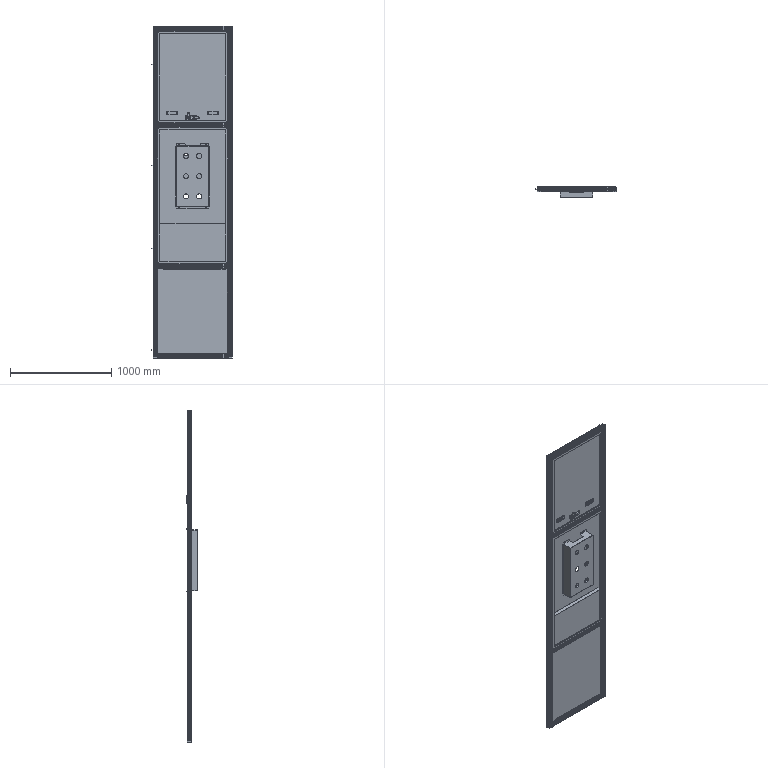Part | SolidWorks | 47 solids | 3133 faces | volume 12397020 mm3 | plane 1903 | cylinder 940 | cone 170 | spline 114 | torus 6 | commonest cylinder face diameters 6.8 x142 2 x92 6.6 x68 20.854 x64 19 x48 10 x43